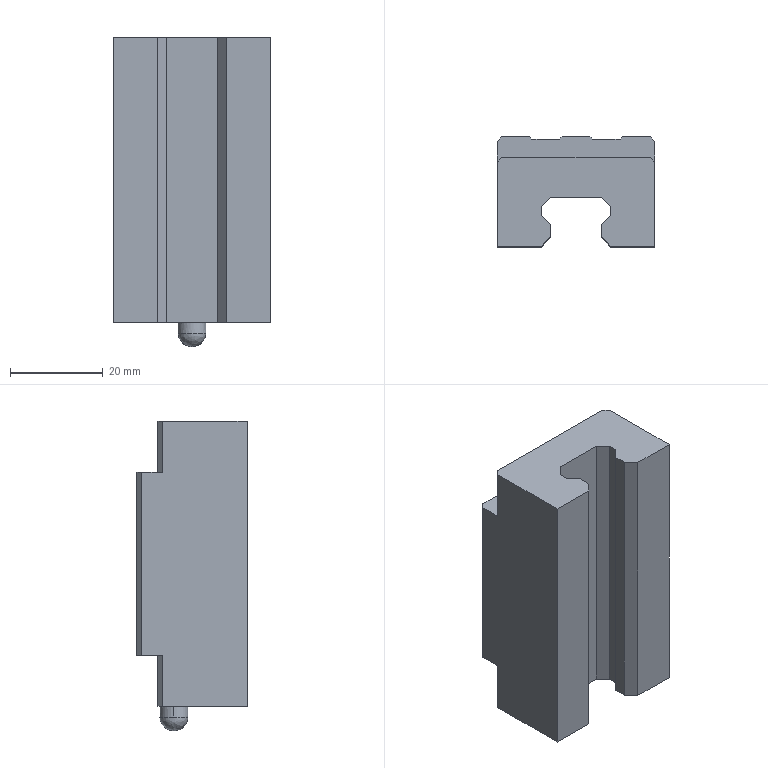Part | SolidWorks | features BaseBody 1 | 1 solid | 55 faces | box 34 x 23.7 x 66.58 mm | volume 37160 mm3 | plane 36 | cylinder 10 | cone 8 | spline 1 | commonest cylinder face diameters 3.242 x8 6 x2